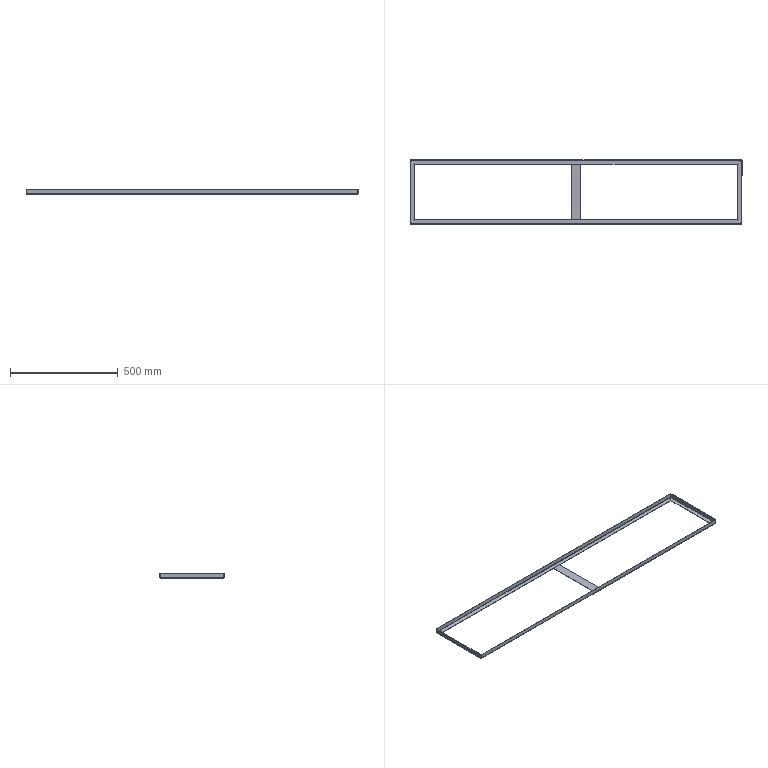Part | STEP file | X77-03012 | 2 solids | 74 faces | box 1538 x 296.5 x 21.5 mm | volume 229108 mm3 | plane 52 | cylinder 14 | spline 8 | commonest cylinder face diameters 1.473 x7 4.473 x7